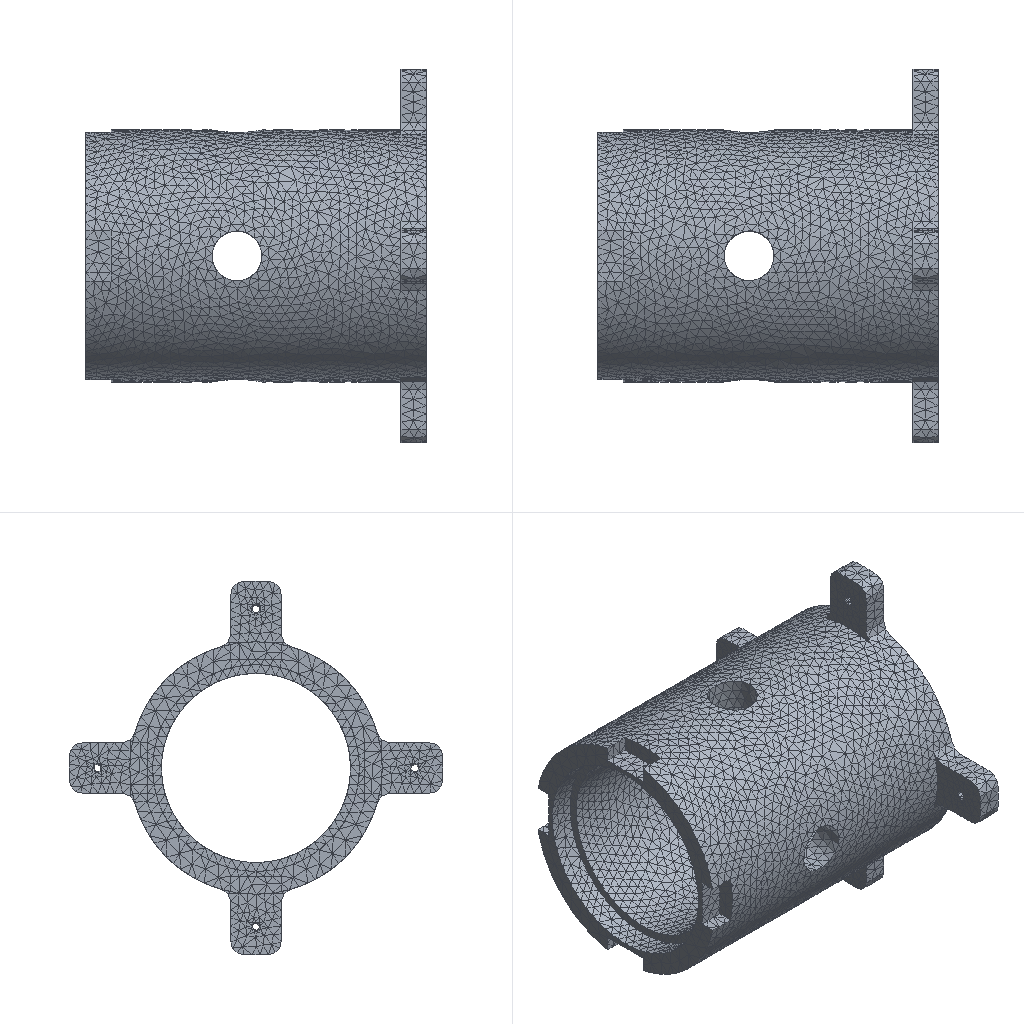Simulation study | ansys workbench
Set-up summary:
category,name,step,type,value,unit,region
solver,ansys_workbench
units,SI m-kg-s (Pa),,stated,"/units,MKS"
analysis,LS1,,static
load_step,LS1,LS1,static,nsubst=1; time=1
mesh,nodes,,,59331
mesh,elements,,,37095
element_type,SOLID187,,,35007
element_type,CONTA174,,,2088
material,Structural Steel,,E,2e+11,Pa
material,Structural Steel,,nu,0.3
material,Structural Steel,,density,7850,kg m^-3
material,Structural Steel,,conductivity,60.5,W m^-1 C^-1
material,Structural Steel,,specific_heat,434,J kg^-1 C^-1
material,Structural Steel,,cte,1.2e-05,C^-1
material,Structural Steel,,permeability,10000
material,Structural Steel,,resistivity,1.7e-07,kg m^3 A^-2 s^-3
load,,LS1,moment,"2000 [dir=(1, 0, 0) n=3]",,all
bc,Fixed Supports,model,fixed,[dofs=ALL],,_FIXEDSU
contact,contact 1,,bonded (always),element=CONTA174
named_set,_FIXEDSU,,node,1477
Ansys APDL input file, long lists of numbers shortened:
/batch
/config,noeldb,1     ! force off writing results to database
*get,_wallstrt,active,,time,wall
! ANSYS input file written by Workbench version 2024 R1
! File used for geometry attach:
/title,wbnew--____ (A5)
! ****** Begin Custom Load Command Snippet ******
/COM, ACT Extensions:
/COM,     LSDYNA, 2024.1
/COM,/COM,     ANSYSMotion, 2024.1
/COM,
! ****** End   Custom Load Command Snippet ******
*DIM,_wb_ProjectScratch_dir,string,248
_wb_ProjectScratch_dir(1) = ''
*DIM,_wb_SolverFiles_dir,string,248
_wb_SolverFiles_dir(1) = ''
*DIM,_wb_userfiles_dir,string,248
_wb_userfiles_dir(1) = ''
/com,--- Data in consistent MKS units. See Solving Units in the help system for more information.
/units,MKS
/nopr
/wb,file,start              !  signify a WB generated input file
/prep7
! Turn off shape checking because checks already performed inside WB mesher.
! See help system for more information.
SHPP,OFF,,NOWARN
/nolist
etcon,set             ! allow ANSYS to choose best KEYOP's for 180x elements, resets any applicable keyopt to MAPDL defaults
/com,*********** Nodes for the whole assembly ***********
nblock,3,,65263
(1i9,3e20.9e3)
        1     7.800000000E-02     4.852200167E-17    -3.750000000E-02
! (59329 more lines like these left out)
-1
/com,*********** Nodes for all Remote Points ***********
nblock,3
(1i9,3e20.9e3)
    59331     4.085153166E-02     3.691149157E-06    -5.113772119E-06
-1
/wb,elem,start            !  set before creation of elements
/com,*********** Elements for Body 1 "2001" ***********
et,1,187
eblock,19,solid,,35007
(19i9)
        1        1        1        1        0        0        0        0       10        0        1     6665     9068     8508     9058    51006    58995    51003    51005
! (70013 more lines like these left out)
-1
/wb,elem,end               !  done creating elements
/com,*********** Send User Defined Coordinate System(s) ***********
csys,0
toffst,273.15,  ! Temperature offset from absolute zero
/com,*********** Set Reference Temperature ***********
tref,22.
/wb,mat,start              !  starting to send materials
/com,*********** Send Materials ***********
Temperature = 'TEMP' ! Temperature
MP,DENS,1,7850,	! kg m^-3
MP,ALPX,1,1.2e-05,	! C^-1
MP,C,1,434,	! J kg^-1 C^-1
MP,KXX,1,60.5,	! W m^-1 C^-1
MP,RSVX,1,1.7e-07,	! kg m^3 A^-2 s^-3
MP,EX,1,200000000000,	! Pa
MP,NUXY,1,0.3,
MP,MURX,1,10000,
/wb,mat,end                !  done sending materials
!************************* Model Summary ********************
!2001,	ç»æé¢,	matid,	1
!************************* End Model Summary ********************
! get the diagonal of the bounding box. Needed later for other things
*get,_xmin,node,,mnloc,x
*get,_ymin,node,,mnloc,y
*get,_zmin,node,,mnloc,z
*get,_xmax,node,,mxloc,x
*get,_ymax,node,,mxloc,y
*get,_zmax,node,,mxloc,z
_ASMDIAG=(_xmax-_xmin)*(_xmax-_xmin)+(_ymax-_ymin)*(_ymax-_ymin)+(_zmax-_zmin)*(_zmax-_zmin)
_ASMDIAG=SQRT(_ASMDIAG)
/wb,contact,start          !  starting to send contact
/wb,contact,end            !  done creating contacts
/golist
/wb,load,start             !  starting to send loads
/com,*********** Fixed Supports ***********
CMBLOCK,_FIXEDSU,NODE,     1477
(8i10)
       371       374       375       376       377       378       379       380
! (184 more lines like these left out)
cmsel,s,_FIXEDSU
d,all,all
nsel,all
/com,*********** Create Remote Point "ÄÚ²¿Ô¶³Ìµã" ***********
! -------- Remote Point Used by "Á¦¾Ø" --------
*set,tid,3
*set,cid,2
et,cid,174
et,tid,170
keyo,tid,2,1               ! Don't fix the pilot node
keyo,tid,4,111111
keyo,cid,12,5              ! Bonded Contact
keyo,cid,4,1               ! Deformable RBE3 style load
keyo,cid,2,2               ! MPC style contact
eblock,10,,,2088
(15i9)
    47355        2        2        2        0       60       61     3810     3810     9421     9430     3810     9424
! (2087 more lines like these left out)
-1
*set,_npilot,59331
_npilot32=_npilot
type,tid
mat ,cid
real,cid
tshape,pilo
en,49443,_npilot
tshape
/com,*********** Construct Moment Using Remote Attachment ***********
/gst,on,on
fini
*get,_numnode,node,0,count
*get,_numelem,elem,0,count
*get, _MAXELEMNUM, elem, 0, NUM, MAX
*get, _MAXNODENUM, node, 0, NUM, MAX
*get, _MAXELEMTYPE, etyp, 0, NUM, MAX
*get, _MAXREALCONST, rcon, 0, NUM, MAX
/go
/wb,load,end               !  done creating loads
/com,--- Number of total nodes = %_numnode%
/com,--- Number of contact elements = 2088
/com,--- Number of spring elements = 0
/com,--- Number of bearing elements = 0
/com,--- Number of solid elements = 35007
/com,--- Number of condensed parts = 0
/com,--- Number of total elements = %_numelem%
*get,_wallbsol,active,,time,wall
/com,****************************************************************************
/com,*************************    SOLUTION       ********************************
/com,****************************************************************************
/solu
antype,0                   ! static analysis
_thickRatio=  1     ! Ratio of thick parts in the model
eqsl,pcg,1e-8,,,,,,1
cntr,print,1               ! print out contact info and also make no initial contact an error
cncheck,dmp		!	Enable program controlled contact splitting for distributed memory parallel run
dmpoption,emat,no             ! Don't combine emat file for DANSYS
dmpoption,esav,no             ! Don't combine esav file for DANSYS
nldiag,cont,iter           ! print out contact info each equilibrium iteration
rescontrol,,none                 ! Do not keep any restart files
/com,****************************************************
/com,******************* SOLVE FOR LS 1 OF 1 ****************
nsel,s,node,,59331
f,all,mx,2000.
f,all,my,0.
f,all,mz,0.
nsel,all
/nopr
/gopr
nsub,1,1,1
time,1.
outres,erase
outres,all,none
outres,nsol,all,
outres,rsol,all
outres,eangl,all
outres,etmp,all
outres,veng,all
outres,strs,all,
outres,epel,all,
outres,eppl,all,
outres,cont,all,
! *********** WB SOLVE COMMAND ***********
! check interactive state
*get,ANSINTER_,active,,int
*if,ANSINTER_,ne,0,then
/eof
*endif
solve
/com *************** Write FE CONNECTORS *********
CEWRITE,file,ce,,INTE
/com,****************************************************
/com,*************** FINISHED SOLVE FOR LS 1 *************
*get,_wallasol,active,,time,wall
/nopr
*get,_numnode,node,0,count
*get,_numelem,elem,0,count
*get, _MAXELEMNUM, elem, 0, NUM, MAX
*get, _MAXNODENUM, node, 0, NUM, MAX,,,INTERNAL
*get, _MAXELEMTYPE, etyp, 0, NUM, MAX
*get, _MAXREALCONST, rcon, 0, NUM, MAX
*get,_NSOLTHREADS,active,0,ntfs
*get,_NSOLPROCESSES,active,0,npfs
/gopr
*get,_PCGITER,active,,solu,cgiter
/post1
xmlo,ENCODING,ISO-8859-1
xmlo,parm
/xml,parm,xml
fini
/gopr
*get,_walldone,active,,time,wall
_preptime=(_wallbsol-_wallstrt)*3600
_solvtime=(_wallasol-_wallbsol)*3600
_posttime=(_walldone-_wallasol)*3600
_totaltim=(_walldone-_wallstrt)*3600
*get,_dlbratio,active,0,solu,dlbr
*get,_combtime,active,0,solu,comb
*get,_ssmode,active,0,solu,ssmm
*get,_ndofs,active,0,solu,ndof
*get,_sol_end_time,active,0,set,time
*if,_sol_end_time,eq,1.,then
/fclean				!clean distributed files
*endif
/com,--- Total number of nodes = %_numnode%
/com,--- Total number of elements = %_numelem%
/com,--- Element load balance ratio = %_dlbratio%
/com,--- Time to combine distributed files = %_combtime%
/com,--- Sparse memory mode = %_ssmode%
/com,--- Number of DOF = %_ndofs%
/wb,file,end               ! done with WB generated input
Results summary:
result,analyses[0].index,,,1
result,analyses[0].system,,,SYS
result,analyses[0].deck,,,deck.dat
result,analyses[0].solve_status,,,completed
result,analyses[0].analysis_type,,,static
result,analyses[0].physics,,,mechanical
result,analyses[0].unit_system,,,"MKS: m, kg, N, s, V, A, degC"
result,analyses[0].n_sets,,,1
result,analyses[0].load_steps[0].set,set=1,,1
result,analyses[0].load_steps[0].time_or_freq,set=1,,1
result,analyses[0].load_steps[0].max_displacement_magnitude,set=1,,2.34398e-05
result,analyses[0].load_steps[0].max_von_mises_nodal,set=1,,4.99104e+07
result,analyses[0].load_steps[0].reaction_force_sum_xyz[1],set=1,,-2.03633e-05
result,analyses[0].load_steps[0].reaction_force_sum_xyz[2],set=1,,1.2382e-05
result,analyses[0].load_steps[0].reaction_force_sum_xyz[3],set=1,,-9.59288e-06
result,geometry_export[0][0],,,.step
result,geometry_export[0][1],,,ok
result,geometry_export[0][2],,,1